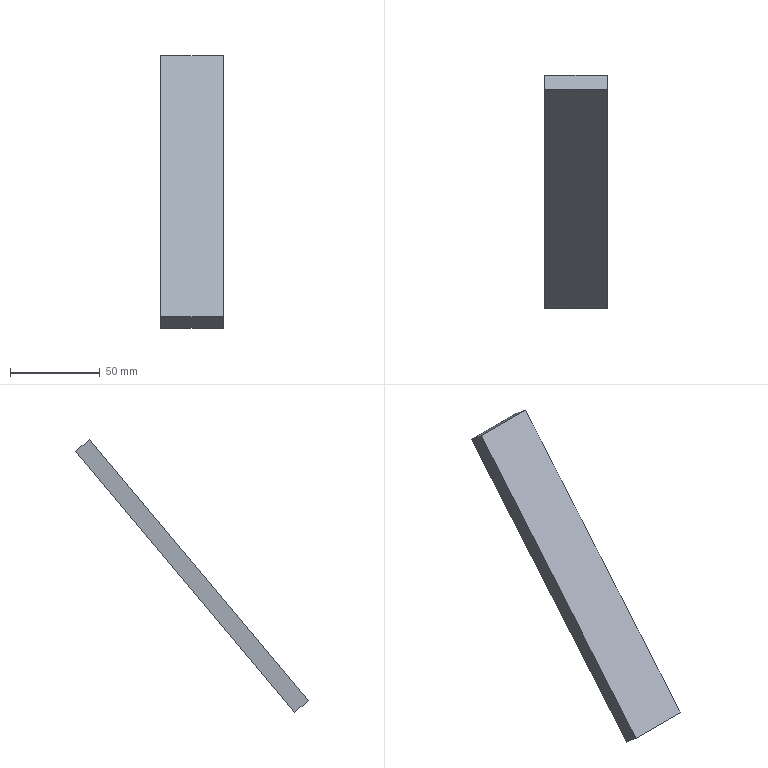Part | NX | features solid 2 | 1 solid | 6 faces | box 35 x 129.79 x 151.976 mm | volume 66500 mm3 | plane 6
STEP:
#1=CARTESIAN_POINT('',(100.,-297.888,-117.268));
#2=VERTEX_POINT('',#1);
#3=CARTESIAN_POINT('',(100.,-305.548,-110.84));
#4=VERTEX_POINT('',#3);
#5=CARTESIAN_POINT('',(100.,-297.888,-117.268));
#6=DIRECTION('',(0.,-0.766,0.6428));
#7=VECTOR('',#6,1000.);
#8=LINE('',#5,#7);
#9=EDGE_CURVE('',#2,#4,#8,.T.);
#10=ORIENTED_EDGE('',*,*,#9,.T.);
#11=CARTESIAN_POINT('',(65.,-305.548,-110.84));
#12=VERTEX_POINT('',#11);
#13=CARTESIAN_POINT('',(65.,-305.548,-110.84));
#14=DIRECTION('',(1.,0.,0.));
#15=VECTOR('',#14,1000.);
#16=LINE('',#13,#15);
#17=EDGE_CURVE('',#12,#4,#16,.T.);
#18=ORIENTED_EDGE('',*,*,#17,.F.);
#19=CARTESIAN_POINT('',(65.,-297.888,-117.268));
#20=VERTEX_POINT('',#19);
#21=CARTESIAN_POINT('',(65.,-297.888,-117.268));
#22=DIRECTION('',(0.,-0.766,0.6428));
#23=VECTOR('',#22,1000.);
#24=LINE('',#21,#23);
#25=EDGE_CURVE('',#20,#12,#24,.T.);
#26=ORIENTED_EDGE('',*,*,#25,.F.);
#27=CARTESIAN_POINT('',(65.,-297.888,-117.268));
#28=DIRECTION('',(1.,0.,0.));
#29=VECTOR('',#28,1000.);
#30=LINE('',#27,#29);
#31=EDGE_CURVE('',#20,#2,#30,.T.);
#32=ORIENTED_EDGE('',*,*,#31,.T.);
#33=EDGE_LOOP('',(#10,#18,#26,#32));
#34=FACE_BOUND('',#33,.T.);
#35=CARTESIAN_POINT('',(65.,-297.888,-117.268));
#36=DIRECTION('',(0.,0.6428,0.766));
#37=DIRECTION('',(0.,0.766,-0.6428));
#38=AXIS2_PLACEMENT_3D('',#35,#36,#37);
#39=PLANE('',#38);
#40=ADVANCED_FACE('',(#34),#39,.F.);
#41=CARTESIAN_POINT('',(100.,-183.418,34.708));
#42=VERTEX_POINT('',#41);
#43=CARTESIAN_POINT('',(100.,-305.548,-110.84));
#44=DIRECTION('',(0.,0.6428,0.766));
#45=VECTOR('',#44,1000.);
#46=LINE('',#43,#45);
#47=EDGE_CURVE('',#4,#42,#46,.T.);
#48=ORIENTED_EDGE('',*,*,#47,.T.);
#49=CARTESIAN_POINT('',(65.,-183.418,34.708));
#50=VERTEX_POINT('',#49);
#51=CARTESIAN_POINT('',(65.,-183.418,34.708));
#52=DIRECTION('',(1.,0.,0.));
#53=VECTOR('',#52,1000.);
#54=LINE('',#51,#53);
#55=EDGE_CURVE('',#50,#42,#54,.T.);
#56=ORIENTED_EDGE('',*,*,#55,.F.);
#57=CARTESIAN_POINT('',(65.,-305.548,-110.84));
#58=DIRECTION('',(0.,0.6428,0.766));
#59=VECTOR('',#58,1000.);
#60=LINE('',#57,#59);
#61=EDGE_CURVE('',#12,#50,#60,.T.);
#62=ORIENTED_EDGE('',*,*,#61,.F.);
#63=ORIENTED_EDGE('',*,*,#17,.T.);
#64=EDGE_LOOP('',(#48,#56,#62,#63));
#65=FACE_BOUND('',#64,.T.);
#66=CARTESIAN_POINT('',(65.,-305.548,-110.84));
#67=DIRECTION('',(0.,0.766,-0.6428));
#68=DIRECTION('',(0.,-0.6428,-0.766));
#69=AXIS2_PLACEMENT_3D('',#66,#67,#68);
#70=PLANE('',#69);
#71=ADVANCED_FACE('',(#65),#70,.F.);
#72=CARTESIAN_POINT('',(100.,-175.758,28.28));
#73=VERTEX_POINT('',#72);
#74=CARTESIAN_POINT('',(100.,-175.758,28.28));
#75=DIRECTION('',(0.,-0.766,0.6428));
#76=VECTOR('',#75,1000.);
#77=LINE('',#74,#76);
#78=EDGE_CURVE('',#73,#42,#77,.T.);
#79=ORIENTED_EDGE('',*,*,#78,.F.);
#80=CARTESIAN_POINT('',(65.,-175.758,28.28));
#81=VERTEX_POINT('',#80);
#82=CARTESIAN_POINT('',(65.,-175.758,28.28));
#83=DIRECTION('',(1.,0.,0.));
#84=VECTOR('',#83,1000.);
#85=LINE('',#82,#84);
#86=EDGE_CURVE('',#81,#73,#85,.T.);
#87=ORIENTED_EDGE('',*,*,#86,.F.);
#88=CARTESIAN_POINT('',(65.,-175.758,28.28));
#89=DIRECTION('',(0.,-0.766,0.6428));
#90=VECTOR('',#89,1000.);
#91=LINE('',#88,#90);
#92=EDGE_CURVE('',#81,#50,#91,.T.);
#93=ORIENTED_EDGE('',*,*,#92,.T.);
#94=ORIENTED_EDGE('',*,*,#55,.T.);
#95=EDGE_LOOP('',(#79,#87,#93,#94));
#96=FACE_BOUND('',#95,.T.);
#97=CARTESIAN_POINT('',(65.,-175.758,28.28));
#98=DIRECTION('',(0.,0.6428,0.766));
#99=DIRECTION('',(0.,0.766,-0.6428));
#100=AXIS2_PLACEMENT_3D('',#97,#98,#99);
#101=PLANE('',#100);
#102=ADVANCED_FACE('',(#96),#101,.T.);
#103=CARTESIAN_POINT('',(100.,-242.461,-51.214));
#104=DIRECTION('',(0.,-0.6428,-0.766));
#105=VECTOR('',#104,1000.);
#106=LINE('',#103,#105);
#107=EDGE_CURVE('',#73,#2,#106,.T.);
#108=ORIENTED_EDGE('',*,*,#107,.T.);
#109=ORIENTED_EDGE('',*,*,#31,.F.);
#110=CARTESIAN_POINT('',(65.,-175.758,28.28));
#111=DIRECTION('',(0.,-0.6428,-0.766));
#112=VECTOR('',#111,1000.);
#113=LINE('',#110,#112);
#114=EDGE_CURVE('',#81,#20,#113,.T.);
#115=ORIENTED_EDGE('',*,*,#114,.F.);
#116=ORIENTED_EDGE('',*,*,#86,.T.);
#117=EDGE_LOOP('',(#108,#109,#115,#116));
#118=FACE_BOUND('',#117,.T.);
#119=CARTESIAN_POINT('',(65.,-242.461,-51.214));
#120=DIRECTION('',(0.,-0.766,0.6428));
#121=DIRECTION('',(0.,0.6428,0.766));
#122=AXIS2_PLACEMENT_3D('',#119,#120,#121);
#123=PLANE('',#122);
#124=ADVANCED_FACE('',(#118),#123,.F.);
#125=ORIENTED_EDGE('',*,*,#25,.T.);
#126=ORIENTED_EDGE('',*,*,#61,.T.);
#127=ORIENTED_EDGE('',*,*,#92,.F.);
#128=ORIENTED_EDGE('',*,*,#114,.T.);
#129=EDGE_LOOP('',(#125,#126,#127,#128));
#130=FACE_BOUND('',#129,.T.);
#131=CARTESIAN_POINT('',(65.,-305.548,-110.84));
#132=DIRECTION('',(-1.,0.,0.));
#133=DIRECTION('',(0.,0.,1.));
#134=AXIS2_PLACEMENT_3D('',#131,#132,#133);
#135=PLANE('',#134);
#136=ADVANCED_FACE('',(#130),#135,.T.);
#137=ORIENTED_EDGE('',*,*,#9,.F.);
#138=ORIENTED_EDGE('',*,*,#107,.F.);
#139=ORIENTED_EDGE('',*,*,#78,.T.);
#140=ORIENTED_EDGE('',*,*,#47,.F.);
#141=EDGE_LOOP('',(#137,#138,#139,#140));
#142=FACE_BOUND('',#141,.T.);
#143=CARTESIAN_POINT('',(100.,-305.548,-110.84));
#144=DIRECTION('',(-1.,0.,0.));
#145=DIRECTION('',(0.,0.,1.));
#146=AXIS2_PLACEMENT_3D('',#143,#144,#145);
#147=PLANE('',#146);
#148=ADVANCED_FACE('',(#142),#147,.F.);
#149=CLOSED_SHELL('',(#40,#71,#102,#124,#136,#148));
#150=MANIFOLD_SOLID_BREP('',#149);
#151=(LENGTH_UNIT()NAMED_UNIT(*)SI_UNIT(.MILLI.,.METRE.));
#152=UNCERTAINTY_MEASURE_WITH_UNIT(LENGTH_MEASURE(0.00001),#151,'','');
#153=(NAMED_UNIT(*)PLANE_ANGLE_UNIT()SI_UNIT($,.RADIAN.));
#154=(NAMED_UNIT(*)SI_UNIT($,.STERADIAN.)SOLID_ANGLE_UNIT());
#155=(GEOMETRIC_REPRESENTATION_CONTEXT(3)GLOBAL_UNCERTAINTY_ASSIGNED_CONTEXT((#152))GLOBAL_UNIT_ASSIGNED_CONTEXT((#151,#153,#154))REPRESENTATION_CONTEXT('',''));
#156=ADVANCED_BREP_SHAPE_REPRESENTATION('',(#150),#155);